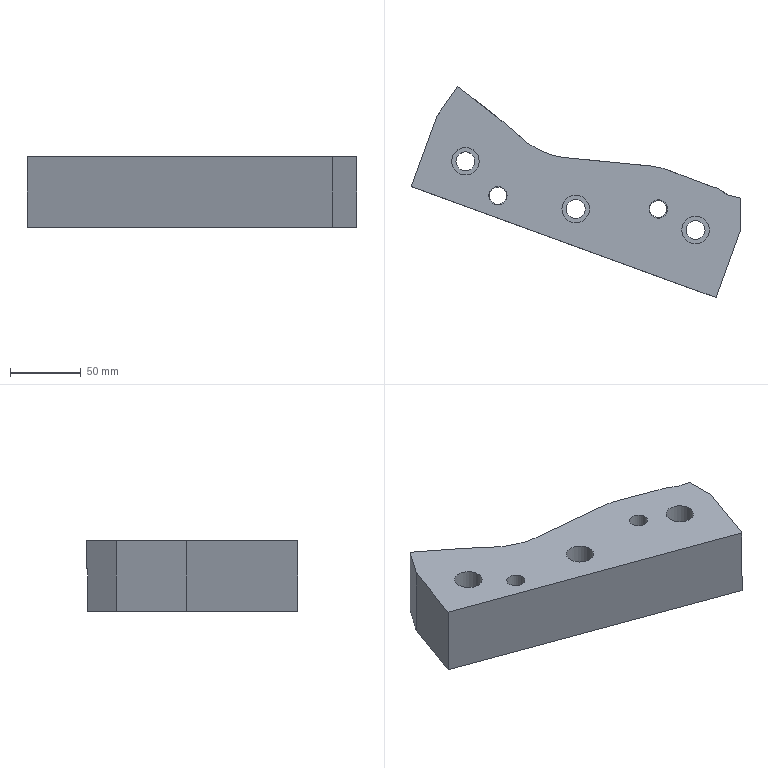Part | NX | features solid 2 | 1 solid | 26 faces | box 233.69 x 149.736 x 50 mm | volume 721253 mm3 | plane 13 | cylinder 10 | spline 3 | commonest cylinder face diameters 13.5 x3 19.5 x3 12 x2 13 x2